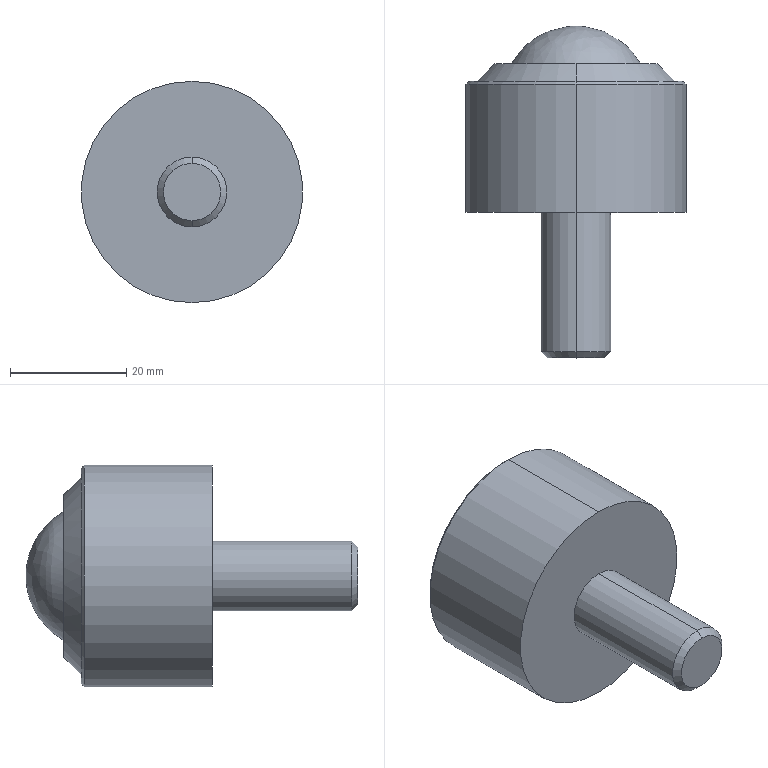Part | SolidWorks | features BaseBody 1 | 1 solid | 15 faces | box 38 x 57 x 38 mm | volume 31976 mm3 | cone 6 | plane 4 | cylinder 4 | spline 1 | commonest cylinder face diameters 12 x2 38 x2
STEP:
#1=CARTESIAN_POINT('',(0.,25.5,11.084));
#2=VERTEX_POINT('',#1);
#3=CARTESIAN_POINT('',(0.003918,25.5,-11.084));
#4=VERTEX_POINT('',#3);
#5=CARTESIAN_POINT('',(0.,25.5,11.084));
#6=CARTESIAN_POINT('',(0.3654,25.5,11.084));
#7=CARTESIAN_POINT('',(0.7294,25.5,11.066));
#8=CARTESIAN_POINT('',(1.27,25.5,11.012));
#9=CARTESIAN_POINT('',(1.45,25.5,10.99));
#10=CARTESIAN_POINT('',(1.718,25.5,10.95));
#11=CARTESIAN_POINT('',(1.851,25.5,10.929));
#12=CARTESIAN_POINT('',(1.984,25.5,10.905));
#13=CARTESIAN_POINT('',(2.072,25.5,10.888));
#14=CARTESIAN_POINT('',(2.115,25.5,10.88));
#15=CARTESIAN_POINT('',(2.526,25.5,10.799));
#16=CARTESIAN_POINT('',(2.883,25.5,10.708));
#17=CARTESIAN_POINT('',(3.405,25.5,10.549));
#18=CARTESIAN_POINT('',(3.576,25.5,10.492));
#19=CARTESIAN_POINT('',(3.83,25.5,10.402));
#20=CARTESIAN_POINT('',(3.955,25.5,10.355));
#21=CARTESIAN_POINT('',(4.1,25.5,10.298));
#22=CARTESIAN_POINT('',(4.162,25.5,10.273));
#23=CARTESIAN_POINT('',(4.203,25.5,10.256));
#24=CARTESIAN_POINT('',(4.222,25.5,10.248));
#25=CARTESIAN_POINT('',(4.592,25.5,10.095));
#26=CARTESIAN_POINT('',(4.926,25.5,9.936));
#27=CARTESIAN_POINT('',(5.403,25.5,9.679));
#28=CARTESIAN_POINT('',(5.559,25.5,9.591));
#29=CARTESIAN_POINT('',(5.786,25.5,9.454));
#30=CARTESIAN_POINT('',(5.898,25.5,9.385));
#31=CARTESIAN_POINT('',(6.027,25.5,9.302));
#32=CARTESIAN_POINT('',(6.091,25.5,9.26));
#33=CARTESIAN_POINT('',(6.118,25.5,9.242));
#34=CARTESIAN_POINT('',(6.136,25.5,9.23));
#35=CARTESIAN_POINT('',(6.144,25.5,9.225));
#36=CARTESIAN_POINT('',(6.474,25.5,9.005));
#37=CARTESIAN_POINT('',(6.774,25.5,8.78));
#38=CARTESIAN_POINT('',(7.194,25.5,8.434));
#39=CARTESIAN_POINT('',(7.33,25.5,8.316));
#40=CARTESIAN_POINT('',(7.525,25.5,8.138));
#41=CARTESIAN_POINT('',(7.622,25.5,8.048));
#42=CARTESIAN_POINT('',(7.731,25.5,7.943));
#43=CARTESIAN_POINT('',(7.785,25.5,7.89));
#44=CARTESIAN_POINT('',(7.808,25.5,7.867));
#45=CARTESIAN_POINT('',(7.823,25.5,7.852));
#46=CARTESIAN_POINT('',(7.83,25.5,7.845));
#47=CARTESIAN_POINT('',(8.112,25.5,7.562));
#48=CARTESIAN_POINT('',(8.362,25.5,7.284));
#49=CARTESIAN_POINT('',(8.704,25.5,6.864));
#50=CARTESIAN_POINT('',(8.813,25.5,6.724));
#51=CARTESIAN_POINT('',(8.969,25.5,6.513));
#52=CARTESIAN_POINT('',(9.045,25.5,6.408));
#53=CARTESIAN_POINT('',(9.13,25.5,6.285));
#54=CARTESIAN_POINT('',(9.172,25.5,6.223));
#55=CARTESIAN_POINT('',(9.19,25.5,6.197));
#56=CARTESIAN_POINT('',(9.202,25.5,6.179));
#57=CARTESIAN_POINT('',(9.206,25.5,6.172));
#58=CARTESIAN_POINT('',(9.431,25.5,5.836));
#59=CARTESIAN_POINT('',(9.622,25.5,5.513));
#60=CARTESIAN_POINT('',(9.877,25.5,5.033));
#61=CARTESIAN_POINT('',(9.956,25.5,4.874));
#62=CARTESIAN_POINT('',(10.068,25.5,4.637));
#63=CARTESIAN_POINT('',(10.122,25.5,4.519));
#64=CARTESIAN_POINT('',(10.181,25.5,4.381));
#65=CARTESIAN_POINT('',(10.211,25.5,4.312));
#66=CARTESIAN_POINT('',(10.223,25.5,4.283));
#67=CARTESIAN_POINT('',(10.231,25.5,4.263));
#68=CARTESIAN_POINT('',(10.234,25.5,4.255));
#69=CARTESIAN_POINT('',(10.388,25.5,3.884));
#70=CARTESIAN_POINT('',(10.512,25.5,3.533));
#71=CARTESIAN_POINT('',(10.668,25.5,3.015));
#72=CARTESIAN_POINT('',(10.714,25.5,2.843));
#73=CARTESIAN_POINT('',(10.778,25.5,2.588));
#74=CARTESIAN_POINT('',(10.808,25.5,2.46));
#75=CARTESIAN_POINT('',(10.84,25.5,2.311));
#76=CARTESIAN_POINT('',(10.853,25.5,2.248));
#77=CARTESIAN_POINT('',(10.862,25.5,2.206));
#78=CARTESIAN_POINT('',(10.866,25.5,2.186));
#79=CARTESIAN_POINT('',(10.907,25.5,1.981));
#80=CARTESIAN_POINT('',(10.938,25.5,1.801));
#81=CARTESIAN_POINT('',(10.978,25.5,1.533));
#82=CARTESIAN_POINT('',(10.99,25.5,1.444));
#83=CARTESIAN_POINT('',(11.012,25.5,1.265));
#84=CARTESIAN_POINT('',(11.021,25.5,1.178));
#85=CARTESIAN_POINT('',(11.066,25.5,0.7244));
#86=CARTESIAN_POINT('',(11.084,25.5,0.3682));
#87=CARTESIAN_POINT('',(11.084,25.5,-0.1753));
#88=CARTESIAN_POINT('',(11.08,25.5,-0.3557));
#89=CARTESIAN_POINT('',(11.066,25.5,-0.627));
#90=CARTESIAN_POINT('',(11.061,25.5,-0.7175));
#91=CARTESIAN_POINT('',(11.048,25.5,-0.899));
#92=CARTESIAN_POINT('',(11.04,25.5,-0.9918));
#93=CARTESIAN_POINT('',(11.013,25.5,-1.26));
#94=CARTESIAN_POINT('',(10.992,25.5,-1.439));
#95=CARTESIAN_POINT('',(10.952,25.5,-1.709));
#96=CARTESIAN_POINT('',(10.93,25.5,-1.844));
#97=CARTESIAN_POINT('',(10.902,25.5,-2.002));
#98=CARTESIAN_POINT('',(10.889,25.5,-2.071));
#99=CARTESIAN_POINT('',(10.88,25.5,-2.116));
#100=CARTESIAN_POINT('',(10.875,25.5,-2.141));
#101=CARTESIAN_POINT('',(10.804,25.5,-2.499));
#102=CARTESIAN_POINT('',(10.72,25.5,-2.838));
#103=CARTESIAN_POINT('',(10.566,25.5,-3.355));
#104=CARTESIAN_POINT('',(10.509,25.5,-3.528));
#105=CARTESIAN_POINT('',(10.416,25.5,-3.791));
#106=CARTESIAN_POINT('',(10.367,25.5,-3.923));
#107=CARTESIAN_POINT('',(10.306,25.5,-4.078));
#108=CARTESIAN_POINT('',(10.275,25.5,-4.156));
#109=CARTESIAN_POINT('',(10.261,25.5,-4.19));
#110=CARTESIAN_POINT('',(10.252,25.5,-4.212));
#111=CARTESIAN_POINT('',(10.247,25.5,-4.225));
#112=CARTESIAN_POINT('',(10.113,25.5,-4.548));
#113=CARTESIAN_POINT('',(9.966,25.5,-4.865));
#114=CARTESIAN_POINT('',(9.711,25.5,-5.345));
#115=CARTESIAN_POINT('',(9.621,25.5,-5.506));
#116=CARTESIAN_POINT('',(9.477,25.5,-5.749));
#117=CARTESIAN_POINT('',(9.402,25.5,-5.87));
#118=CARTESIAN_POINT('',(9.311,25.5,-6.013));
#119=CARTESIAN_POINT('',(9.265,25.5,-6.084));
#120=CARTESIAN_POINT('',(9.245,25.5,-6.115));
#121=CARTESIAN_POINT('',(9.231,25.5,-6.135));
#122=CARTESIAN_POINT('',(9.223,25.5,-6.147));
#123=CARTESIAN_POINT('',(9.029,25.5,-6.437));
#124=CARTESIAN_POINT('',(8.823,25.5,-6.719));
#125=CARTESIAN_POINT('',(8.48,25.5,-7.139));
#126=CARTESIAN_POINT('',(8.361,25.5,-7.279));
#127=CARTESIAN_POINT('',(8.173,25.5,-7.488));
#128=CARTESIAN_POINT('',(8.076,25.5,-7.592));
#129=CARTESIAN_POINT('',(7.96,25.5,-7.713));
#130=CARTESIAN_POINT('',(7.901,25.5,-7.773));
#131=CARTESIAN_POINT('',(7.876,25.5,-7.799));
#132=CARTESIAN_POINT('',(7.859,25.5,-7.816));
#133=CARTESIAN_POINT('',(7.849,25.5,-7.826));
#134=CARTESIAN_POINT('',(7.599,25.5,-8.076));
#135=CARTESIAN_POINT('',(7.34,25.5,-8.313));
#136=CARTESIAN_POINT('',(6.921,25.5,-8.66));
#137=CARTESIAN_POINT('',(6.776,25.5,-8.773));
#138=CARTESIAN_POINT('',(6.552,25.5,-8.94));
#139=CARTESIAN_POINT('',(6.438,25.5,-9.023));
#140=CARTESIAN_POINT('',(6.302,25.5,-9.118));
#141=CARTESIAN_POINT('',(6.243,25.5,-9.159));
#142=CARTESIAN_POINT('',(6.203,25.5,-9.185));
#143=CARTESIAN_POINT('',(6.181,25.5,-9.2));
#144=CARTESIAN_POINT('',(5.874,25.5,-9.406));
#145=CARTESIAN_POINT('',(5.569,25.5,-9.59));
#146=CARTESIAN_POINT('',(5.089,25.5,-9.848));
#147=CARTESIAN_POINT('',(4.926,25.5,-9.931));
#148=CARTESIAN_POINT('',(4.674,25.5,-10.05));
#149=CARTESIAN_POINT('',(4.547,25.5,-10.109));
#150=CARTESIAN_POINT('',(4.396,25.5,-10.175));
#151=CARTESIAN_POINT('',(4.331,25.5,-10.202));
#152=CARTESIAN_POINT('',(4.288,25.5,-10.221));
#153=CARTESIAN_POINT('',(4.265,25.5,-10.231));
#154=CARTESIAN_POINT('',(3.919,25.5,-10.374));
#155=CARTESIAN_POINT('',(3.583,25.5,-10.495));
#156=CARTESIAN_POINT('',(3.064,25.5,-10.653));
#157=CARTESIAN_POINT('',(2.888,25.5,-10.702));
#158=CARTESIAN_POINT('',(2.622,25.5,-10.77));
#159=CARTESIAN_POINT('',(2.488,25.5,-10.802));
#160=CARTESIAN_POINT('',(2.353,25.5,-10.831));
#161=CARTESIAN_POINT('',(2.263,25.5,-10.85));
#162=CARTESIAN_POINT('',(2.216,25.5,-10.86));
#163=CARTESIAN_POINT('',(1.465,25.5,-11.01));
#164=CARTESIAN_POINT('',(0.7373,25.5,-11.084));
#165=CARTESIAN_POINT('',(0.003918,25.5,-11.084));
#166=B_SPLINE_CURVE_WITH_KNOTS('',3,(#5,#6,#7,#8,#9,#10,#11,#12,#13,#14,#15,#16,#17,#18,#19,#20,#21,#22,#23,#24,#25,#26,#27,#28,#29,#30,#31,#32,#33,#34,#35,#36,#37,#38,#39,#40,#41,#42,#43,#44,#45,#46,#47,#48,#49,#50,#51,#52,#53,#54,#55,#56,#57,#58,#59,#60,#61,#62,#63,#64,#65,#66,#67,#68,#69,#70,#71,#72,#73,#74,#75,#76,#77,#78,#79,#80,#81,#82,#83,#84,#85,#86,#87,#88,#89,#90,#91,#92,#93,#94,#95,#96,#97,#98,#99,#100,#101,#102,#103,#104,#105,#106,#107,#108,#109,#110,#111,#112,#113,#114,#115,#116,#117,#118,#119,#120,#121,#122,#123,#124,#125,#126,#127,#128,#129,#130,#131,#132,#133,#134,#135,#136,#137,#138,#139,#140,#141,#142,#143,#144,#145,#146,#147,#148,#149,#150,#151,#152,#153,#154,#155,#156,#157,#158,#159,#160,#161,#162,#163,#164,#165),.UNSPECIFIED.,.F.,.F.,(4,2,2,1,2,2,2,2,1,1,2,2,2,2,1,1,1,2,2,2,2,1,1,1,2,2,2,2,1,1,1,2,2,2,2,1,1,1,2,2,2,2,1,1,2,2,2,2,2,2,2,2,2,2,1,1,2,2,2,2,1,1,1,2,2,2,2,1,1,1,2,2,2,2,1,1,1,2,2,2,2,1,1,2,2,2,2,1,1,2,2,2,2,1,2,2,4),(0.,0.03125,0.04687,0.05469,0.05859,0.0625,0.09375,0.1094,0.1172,0.1211,0.123,0.125,0.1562,0.1719,0.1797,0.1836,0.1855,0.1865,0.1875,0.2187,0.2344,0.2422,0.2461,0.248,0.249,0.25,0.2812,0.2969,0.3047,0.3086,0.3105,0.3115,0.3125,0.3437,0.3594,0.3672,0.3711,0.373,0.374,0.375,0.4062,0.4219,0.4297,0.4336,0.4355,0.4375,0.4531,0.4609,0.4687,0.5,0.5156,0.5234,0.5312,0.5469,0.5547,0.5586,0.5605,0.5625,0.5937,0.6094,0.6172,0.6211,0.623,0.624,0.625,0.6562,0.6719,0.6797,0.6836,0.6855,0.6865,0.6875,0.7187,0.7344,0.7422,0.7461,0.748,0.749,0.75,0.7812,0.7969,0.8047,0.8086,0.8105,0.8125,0.8437,0.8594,0.8672,0.8711,0.873,0.875,0.9062,0.9219,0.9297,0.9336,0.9375,1.),.UNSPECIFIED.);
#167=EDGE_CURVE('',#2,#4,#166,.T.);
#168=ORIENTED_EDGE('',*,*,#167,.T.);
#169=CARTESIAN_POINT('',(0.003918,25.5,-11.084));
#170=CARTESIAN_POINT('',(-0.3607,25.5,-11.084));
#171=CARTESIAN_POINT('',(-0.7241,25.5,-11.066));
#172=CARTESIAN_POINT('',(-1.264,25.5,-11.013));
#173=CARTESIAN_POINT('',(-1.443,25.5,-10.991));
#174=CARTESIAN_POINT('',(-1.711,25.5,-10.951));
#175=CARTESIAN_POINT('',(-1.844,25.5,-10.93));
#176=CARTESIAN_POINT('',(-1.976,25.5,-10.906));
#177=CARTESIAN_POINT('',(-2.065,25.5,-10.89));
#178=CARTESIAN_POINT('',(-2.107,25.5,-10.882));
#179=CARTESIAN_POINT('',(-2.518,25.5,-10.8));
#180=CARTESIAN_POINT('',(-2.875,25.5,-10.711));
#181=CARTESIAN_POINT('',(-3.396,25.5,-10.552));
#182=CARTESIAN_POINT('',(-3.568,25.5,-10.495));
#183=CARTESIAN_POINT('',(-3.821,25.5,-10.405));
#184=CARTESIAN_POINT('',(-3.946,25.5,-10.358));
#185=CARTESIAN_POINT('',(-4.091,25.5,-10.301));
#186=CARTESIAN_POINT('',(-4.153,25.5,-10.276));
#187=CARTESIAN_POINT('',(-4.194,25.5,-10.26));
#188=CARTESIAN_POINT('',(-4.213,25.5,-10.252));
#189=CARTESIAN_POINT('',(-4.585,25.5,-10.098));
#190=CARTESIAN_POINT('',(-4.919,25.5,-9.939));
#191=CARTESIAN_POINT('',(-5.399,25.5,-9.682));
#192=CARTESIAN_POINT('',(-5.555,25.5,-9.593));
#193=CARTESIAN_POINT('',(-5.783,25.5,-9.456));
#194=CARTESIAN_POINT('',(-5.896,25.5,-9.386));
#195=CARTESIAN_POINT('',(-6.025,25.5,-9.303));
#196=CARTESIAN_POINT('',(-6.08,25.5,-9.267));
#197=CARTESIAN_POINT('',(-6.116,25.5,-9.243));
#198=CARTESIAN_POINT('',(-6.133,25.5,-9.233));
#199=CARTESIAN_POINT('',(-6.471,25.5,-9.007));
#200=CARTESIAN_POINT('',(-6.77,25.5,-8.784));
#201=CARTESIAN_POINT('',(-7.188,25.5,-8.439));
#202=CARTESIAN_POINT('',(-7.323,25.5,-8.322));
#203=CARTESIAN_POINT('',(-7.518,25.5,-8.145));
#204=CARTESIAN_POINT('',(-7.614,25.5,-8.055));
#205=CARTESIAN_POINT('',(-7.723,25.5,-7.95));
#206=CARTESIAN_POINT('',(-7.777,25.5,-7.898));
#207=CARTESIAN_POINT('',(-7.799,25.5,-7.875));
#208=CARTESIAN_POINT('',(-7.815,25.5,-7.86));
#209=CARTESIAN_POINT('',(-7.821,25.5,-7.854));
#210=CARTESIAN_POINT('',(-8.106,25.5,-7.57));
#211=CARTESIAN_POINT('',(-8.357,25.5,-7.29));
#212=CARTESIAN_POINT('',(-8.701,25.5,-6.868));
#213=CARTESIAN_POINT('',(-8.811,25.5,-6.727));
#214=CARTESIAN_POINT('',(-8.967,25.5,-6.515));
#215=CARTESIAN_POINT('',(-9.043,25.5,-6.41));
#216=CARTESIAN_POINT('',(-9.129,25.5,-6.286));
#217=CARTESIAN_POINT('',(-9.171,25.5,-6.224));
#218=CARTESIAN_POINT('',(-9.189,25.5,-6.198));
#219=CARTESIAN_POINT('',(-9.201,25.5,-6.18));
#220=CARTESIAN_POINT('',(-9.206,25.5,-6.173));
#221=CARTESIAN_POINT('',(-9.43,25.5,-5.838));
#222=CARTESIAN_POINT('',(-9.62,25.5,-5.516));
#223=CARTESIAN_POINT('',(-9.874,25.5,-5.039));
#224=CARTESIAN_POINT('',(-9.953,25.5,-4.881));
#225=CARTESIAN_POINT('',(-10.064,25.5,-4.645));
#226=CARTESIAN_POINT('',(-10.118,25.5,-4.527));
#227=CARTESIAN_POINT('',(-10.178,25.5,-4.39));
#228=CARTESIAN_POINT('',(-10.207,25.5,-4.322));
#229=CARTESIAN_POINT('',(-10.219,25.5,-4.292));
#230=CARTESIAN_POINT('',(-10.227,25.5,-4.273));
#231=CARTESIAN_POINT('',(-10.231,25.5,-4.265));
#232=CARTESIAN_POINT('',(-10.385,25.5,-3.893));
#233=CARTESIAN_POINT('',(-10.509,25.5,-3.542));
#234=CARTESIAN_POINT('',(-10.665,25.5,-3.023));
#235=CARTESIAN_POINT('',(-10.712,25.5,-2.851));
#236=CARTESIAN_POINT('',(-10.776,25.5,-2.595));
#237=CARTESIAN_POINT('',(-10.806,25.5,-2.467));
#238=CARTESIAN_POINT('',(-10.839,25.5,-2.318));
#239=CARTESIAN_POINT('',(-10.852,25.5,-2.255));
#240=CARTESIAN_POINT('',(-10.861,25.5,-2.212));
#241=CARTESIAN_POINT('',(-10.865,25.5,-2.193));
#242=CARTESIAN_POINT('',(-10.905,25.5,-1.989));
#243=CARTESIAN_POINT('',(-10.937,25.5,-1.81));
#244=CARTESIAN_POINT('',(-10.976,25.5,-1.542));
#245=CARTESIAN_POINT('',(-10.995,25.5,-1.409));
#246=CARTESIAN_POINT('',(-11.01,25.5,-1.276));
#247=CARTESIAN_POINT('',(-11.02,25.5,-1.188));
#248=CARTESIAN_POINT('',(-11.025,25.5,-1.145));
#249=CARTESIAN_POINT('',(-11.066,25.5,-0.7339));
#250=CARTESIAN_POINT('',(-11.083,25.5,-0.3748));
#251=CARTESIAN_POINT('',(-11.084,25.5,0.1704));
#252=CARTESIAN_POINT('',(-11.08,25.5,0.3515));
#253=CARTESIAN_POINT('',(-11.067,25.5,0.6236));
#254=CARTESIAN_POINT('',(-11.058,25.5,0.7598));
#255=CARTESIAN_POINT('',(-11.048,25.5,0.8965));
#256=CARTESIAN_POINT('',(-11.04,25.5,0.9878));
#257=CARTESIAN_POINT('',(-11.035,25.5,1.035));
#258=CARTESIAN_POINT('',(-11.014,25.5,1.257));
#259=CARTESIAN_POINT('',(-10.992,25.5,1.434));
#260=CARTESIAN_POINT('',(-10.953,25.5,1.702));
#261=CARTESIAN_POINT('',(-10.931,25.5,1.836));
#262=CARTESIAN_POINT('',(-10.903,25.5,1.993));
#263=CARTESIAN_POINT('',(-10.891,25.5,2.061));
#264=CARTESIAN_POINT('',(-10.882,25.5,2.106));
#265=CARTESIAN_POINT('',(-10.877,25.5,2.13));
#266=CARTESIAN_POINT('',(-10.806,25.5,2.49));
#267=CARTESIAN_POINT('',(-10.723,25.5,2.831));
#268=CARTESIAN_POINT('',(-10.567,25.5,3.35));
#269=CARTESIAN_POINT('',(-10.51,25.5,3.524));
#270=CARTESIAN_POINT('',(-10.417,25.5,3.788));
#271=CARTESIAN_POINT('',(-10.368,25.5,3.921));
#272=CARTESIAN_POINT('',(-10.307,25.5,4.077));
#273=CARTESIAN_POINT('',(-10.275,25.5,4.155));
#274=CARTESIAN_POINT('',(-10.262,25.5,4.189));
#275=CARTESIAN_POINT('',(-10.252,25.5,4.212));
#276=CARTESIAN_POINT('',(-10.247,25.5,4.224));
#277=CARTESIAN_POINT('',(-10.114,25.5,4.546));
#278=CARTESIAN_POINT('',(-9.967,25.5,4.861));
#279=CARTESIAN_POINT('',(-9.715,25.5,5.339));
#280=CARTESIAN_POINT('',(-9.625,25.5,5.5));
#281=CARTESIAN_POINT('',(-9.482,25.5,5.741));
#282=CARTESIAN_POINT('',(-9.408,25.5,5.862));
#283=CARTESIAN_POINT('',(-9.317,25.5,6.004));
#284=CARTESIAN_POINT('',(-9.271,25.5,6.075));
#285=CARTESIAN_POINT('',(-9.251,25.5,6.105));
#286=CARTESIAN_POINT('',(-9.237,25.5,6.125));
#287=CARTESIAN_POINT('',(-9.23,25.5,6.137));
#288=CARTESIAN_POINT('',(-9.035,25.5,6.428));
#289=CARTESIAN_POINT('',(-8.828,25.5,6.712));
#290=CARTESIAN_POINT('',(-8.485,25.5,7.134));
#291=CARTESIAN_POINT('',(-8.365,25.5,7.274));
#292=CARTESIAN_POINT('',(-8.176,25.5,7.484));
#293=CARTESIAN_POINT('',(-8.079,25.5,7.589));
#294=CARTESIAN_POINT('',(-7.963,25.5,7.71));
#295=CARTESIAN_POINT('',(-7.904,25.5,7.771));
#296=CARTESIAN_POINT('',(-7.878,25.5,7.797));
#297=CARTESIAN_POINT('',(-7.861,25.5,7.814));
#298=CARTESIAN_POINT('',(-7.851,25.5,7.824));
#299=CARTESIAN_POINT('',(-7.602,25.5,8.073));
#300=CARTESIAN_POINT('',(-7.343,25.5,8.31));
#301=CARTESIAN_POINT('',(-6.926,25.5,8.656));
#302=CARTESIAN_POINT('',(-6.781,25.5,8.769));
#303=CARTESIAN_POINT('',(-6.558,25.5,8.936));
#304=CARTESIAN_POINT('',(-6.444,25.5,9.019));
#305=CARTESIAN_POINT('',(-6.309,25.5,9.114));
#306=CARTESIAN_POINT('',(-6.25,25.5,9.154));
#307=CARTESIAN_POINT('',(-6.21,25.5,9.181));
#308=CARTESIAN_POINT('',(-6.189,25.5,9.195));
#309=CARTESIAN_POINT('',(-5.881,25.5,9.401));
#310=CARTESIAN_POINT('',(-5.577,25.5,9.585));
#311=CARTESIAN_POINT('',(-5.097,25.5,9.844));
#312=CARTESIAN_POINT('',(-4.934,25.5,9.927));
#313=CARTESIAN_POINT('',(-4.683,25.5,10.047));
#314=CARTESIAN_POINT('',(-4.556,25.5,10.105));
#315=CARTESIAN_POINT('',(-4.405,25.5,10.171));
#316=CARTESIAN_POINT('',(-4.34,25.5,10.199));
#317=CARTESIAN_POINT('',(-4.296,25.5,10.217));
#318=CARTESIAN_POINT('',(-4.273,25.5,10.227));
#319=CARTESIAN_POINT('',(-3.926,25.5,10.371));
#320=CARTESIAN_POINT('',(-3.589,25.5,10.493));
#321=CARTESIAN_POINT('',(-3.069,25.5,10.652));
#322=CARTESIAN_POINT('',(-2.893,25.5,10.701));
#323=CARTESIAN_POINT('',(-2.626,25.5,10.769));
#324=CARTESIAN_POINT('',(-2.491,25.5,10.801));
#325=CARTESIAN_POINT('',(-2.356,25.5,10.831));
#326=CARTESIAN_POINT('',(-2.265,25.5,10.85));
#327=CARTESIAN_POINT('',(-2.218,25.5,10.86));
#328=CARTESIAN_POINT('',(-1.465,25.5,11.01));
#329=CARTESIAN_POINT('',(-0.7354,25.5,11.084));
#330=CARTESIAN_POINT('',(0.,25.5,11.084));
#331=B_SPLINE_CURVE_WITH_KNOTS('',3,(#169,#170,#171,#172,#173,#174,#175,#176,#177,#178,#179,#180,#181,#182,#183,#184,#185,#186,#187,#188,#189,#190,#191,#192,#193,#194,#195,#196,#197,#198,#199,#200,#201,#202,#203,#204,#205,#206,#207,#208,#209,#210,#211,#212,#213,#214,#215,#216,#217,#218,#219,#220,#221,#222,#223,#224,#225,#226,#227,#228,#229,#230,#231,#232,#233,#234,#235,#236,#237,#238,#239,#240,#241,#242,#243,#244,#245,#246,#247,#248,#249,#250,#251,#252,#253,#254,#255,#256,#257,#258,#259,#260,#261,#262,#263,#264,#265,#266,#267,#268,#269,#270,#271,#272,#273,#274,#275,#276,#277,#278,#279,#280,#281,#282,#283,#284,#285,#286,#287,#288,#289,#290,#291,#292,#293,#294,#295,#296,#297,#298,#299,#300,#301,#302,#303,#304,#305,#306,#307,#308,#309,#310,#311,#312,#313,#314,#315,#316,#317,#318,#319,#320,#321,#322,#323,#324,#325,#326,#327,#328,#329,#330),.UNSPECIFIED.,.F.,.F.,(4,2,2,1,2,2,2,2,1,1,2,2,2,2,1,1,2,2,2,2,1,1,1,2,2,2,2,1,1,1,2,2,2,2,1,1,1,2,2,2,2,1,1,2,2,2,1,2,2,2,2,1,2,2,2,1,1,2,2,2,2,1,1,1,2,2,2,2,1,1,1,2,2,2,2,1,1,1,2,2,2,2,1,1,2,2,2,2,1,1,2,2,2,2,1,2,2,4),(0.,0.03125,0.04687,0.05469,0.05859,0.0625,0.09375,0.1094,0.1172,0.1211,0.123,0.125,0.1563,0.1719,0.1797,0.1836,0.1855,0.1875,0.2188,0.2344,0.2422,0.2461,0.248,0.249,0.25,0.2813,0.2969,0.3047,0.3086,0.3105,0.3115,0.3125,0.3438,0.3594,0.3672,0.3711,0.373,0.374,0.375,0.4063,0.4219,0.4297,0.4336,0.4355,0.4375,0.4531,0.4609,0.4648,0.4688,0.5,0.5156,0.5234,0.5273,0.5313,0.5469,0.5547,0.5586,0.5605,0.5625,0.5938,0.6094,0.6172,0.6211,0.623,0.624,0.625,0.6563,0.6719,0.6797,0.6836,0.6855,0.6865,0.6875,0.7188,0.7344,0.7422,0.7461,0.748,0.749,0.75,0.7813,0.7969,0.8047,0.8086,0.8105,0.8125,0.8438,0.8594,0.8672,0.8711,0.873,0.875,0.9063,0.9219,0.9297,0.9336,0.9375,1.),.UNSPECIFIED.);
#332=EDGE_CURVE('',#4,#2,#331,.T.);
#333=ORIENTED_EDGE('',*,*,#332,.T.);
#334=EDGE_LOOP('',(#168,#333));
#335=FACE_OUTER_BOUND('',#334,.T.);
#336=CARTESIAN_POINT('',(-11.175,22.179,5.304));
#337=CARTESIAN_POINT('',(-11.175,26.959,2.709));
#338=CARTESIAN_POINT('',(-11.175,26.952,-2.73));
#339=CARTESIAN_POINT('',(-11.175,22.164,-5.311));
#340=CARTESIAN_POINT('',(-5.695,27.019,14.222));
#341=CARTESIAN_POINT('',(-5.695,39.837,7.265));
#342=CARTESIAN_POINT('',(-5.695,39.817,-7.32));
#343=CARTESIAN_POINT('',(-5.695,26.981,-14.242));
#344=CARTESIAN_POINT('',(5.836,26.995,14.177));
#345=CARTESIAN_POINT('',(5.836,39.773,7.242));
#346=CARTESIAN_POINT('',(5.836,39.753,-7.297));
#347=CARTESIAN_POINT('',(5.836,26.957,-14.198));
#348=CARTESIAN_POINT('',(11.227,22.132,5.218));
#349=CARTESIAN_POINT('',(11.227,26.835,2.665));
#350=CARTESIAN_POINT('',(11.227,26.828,-2.686));
#351=CARTESIAN_POINT('',(11.227,22.118,-5.225));
#352=(BOUNDED_SURFACE()B_SPLINE_SURFACE(3,3,((#336,#337,#338,#339),(#340,#341,#342,#343),(#344,#345,#346,#347),(#348,#349,#350,#351)),.UNSPECIFIED.,.F.,.F.,.F.)B_SPLINE_SURFACE_WITH_KNOTS((4,4),(4,4),(0.,1.),(0.,1.),.UNSPECIFIED.)GEOMETRIC_REPRESENTATION_ITEM()RATIONAL_B_SPLINE_SURFACE(((1.,0.6506,0.6506,1.),(0.6475,0.4213,0.4213,0.6475),(0.6475,0.4213,0.4213,0.6475),(1.,0.6506,0.6506,1.)))REPRESENTATION_ITEM('')SURFACE());
#353=ADVANCED_FACE('',(#335),#352,.T.);
#354=ORIENTED_EDGE('',*,*,#167,.F.);
#355=ORIENTED_EDGE('',*,*,#332,.F.);
#356=EDGE_LOOP('',(#354,#355));
#357=FACE_BOUND('',#356,.T.);
#358=CARTESIAN_POINT('',(0.,25.5,-14.));
#359=VERTEX_POINT('',#358);
#360=CARTESIAN_POINT('',(0.,25.5,14.));
#361=VERTEX_POINT('',#360);
#362=CARTESIAN_POINT('',(0.,25.5,0.));
#363=DIRECTION('',(0.,-1.,0.));
#364=DIRECTION('',(0.,0.,-1.));
#365=AXIS2_PLACEMENT_3D('',#362,#363,#364);
#366=CIRCLE('',#365,14.);
#367=EDGE_CURVE('',#359,#361,#366,.T.);
#368=ORIENTED_EDGE('',*,*,#367,.F.);
#369=CARTESIAN_POINT('',(0.,25.5,0.));
#370=DIRECTION('',(0.,-1.,0.));
#371=DIRECTION('',(0.,0.,-1.));
#372=AXIS2_PLACEMENT_3D('',#369,#370,#371);
#373=CIRCLE('',#372,14.);
#374=EDGE_CURVE('',#361,#359,#373,.T.);
#375=ORIENTED_EDGE('',*,*,#374,.F.);
#376=EDGE_LOOP('',(#368,#375));
#377=FACE_OUTER_BOUND('',#376,.T.);
#378=CARTESIAN_POINT('',(-14.,25.5,0.));
#379=DIRECTION('',(0.,-1.,0.));
#380=DIRECTION('',(0.,0.,-1.));
#381=AXIS2_PLACEMENT_3D('',#378,#379,#380);
#382=PLANE('',#381);
#383=ADVANCED_FACE('',(#357,#377),#382,.F.);
#384=CARTESIAN_POINT('',(0.,-25.,4.927));
#385=VERTEX_POINT('',#384);
#386=CARTESIAN_POINT('',(0.,-25.,-4.927));
#387=VERTEX_POINT('',#386);
#388=CARTESIAN_POINT('',(0.,-25.,0.));
#389=DIRECTION('',(0.,1.,0.));
#390=DIRECTION('',(0.,0.,1.));
#391=AXIS2_PLACEMENT_3D('',#388,#389,#390);
#392=CIRCLE('',#391,4.927);
#393=EDGE_CURVE('',#385,#387,#392,.T.);
#394=ORIENTED_EDGE('',*,*,#393,.F.);
#395=CARTESIAN_POINT('',(0.,-25.,0.));
#396=DIRECTION('',(0.,1.,0.));
#397=DIRECTION('',(0.,0.,1.));
#398=AXIS2_PLACEMENT_3D('',#395,#396,#397);
#399=CIRCLE('',#398,4.927);
#400=EDGE_CURVE('',#387,#385,#399,.T.);
#401=ORIENTED_EDGE('',*,*,#400,.F.);
#402=EDGE_LOOP('',(#394,#401));
#403=FACE_OUTER_BOUND('',#402,.T.);
#404=CARTESIAN_POINT('',(0.,-25.,0.));
#405=DIRECTION('',(0.,1.,0.));
#406=DIRECTION('',(1.,0.,0.));
#407=AXIS2_PLACEMENT_3D('',#404,#405,#406);
#408=PLANE('',#407);
#409=ADVANCED_FACE('',(#403),#408,.F.);
#410=CARTESIAN_POINT('',(0.,22.5,17.));
#411=VERTEX_POINT('',#410);
#412=CARTESIAN_POINT('',(0.,22.5,17.));
#413=DIRECTION('',(0.,-0.7071,0.7071));
#414=VECTOR('',#413,1000.);
#415=LINE('',#412,#414);
#416=EDGE_CURVE('',#361,#411,#415,.T.);
#417=ORIENTED_EDGE('',*,*,#416,.F.);
#418=ORIENTED_EDGE('',*,*,#374,.T.);
#419=CARTESIAN_POINT('',(0.,22.5,-17.));
#420=VERTEX_POINT('',#419);
#421=CARTESIAN_POINT('',(0.,22.5,-17.));
#422=DIRECTION('',(0.,-0.7071,-0.7071));
#423=VECTOR('',#422,1000.);
#424=LINE('',#421,#423);
#425=EDGE_CURVE('',#359,#420,#424,.T.);
#426=ORIENTED_EDGE('',*,*,#425,.T.);
#427=CARTESIAN_POINT('',(0.,22.5,0.));
#428=DIRECTION('',(0.,1.,0.));
#429=DIRECTION('',(0.,0.,-1.));
#430=AXIS2_PLACEMENT_3D('',#427,#428,#429);
#431=CIRCLE('',#430,17.);
#432=EDGE_CURVE('',#420,#411,#431,.T.);
#433=ORIENTED_EDGE('',*,*,#432,.T.);
#434=EDGE_LOOP('',(#417,#418,#426,#433));
#435=FACE_OUTER_BOUND('',#434,.T.);
#436=CARTESIAN_POINT('',(0.,22.5,0.));
#437=DIRECTION('',(0.,-1.,0.));
#438=DIRECTION('',(0.,0.,-1.));
#439=AXIS2_PLACEMENT_3D('',#436,#437,#438);
#440=CONICAL_SURFACE('',#439,17.,0.7854);
#441=ADVANCED_FACE('',(#435),#440,.T.);
#442=CARTESIAN_POINT('',(0.,-23.927,-6.));
#443=VERTEX_POINT('',#442);
#444=CARTESIAN_POINT('',(0.,-23.926,-6.));
#445=DIRECTION('',(0.,0.7071,-0.7071));
#446=VECTOR('',#445,1000.);
#447=LINE('',#444,#446);
#448=EDGE_CURVE('',#387,#443,#447,.T.);
#449=ORIENTED_EDGE('',*,*,#448,.F.);
#450=ORIENTED_EDGE('',*,*,#400,.T.);
#451=CARTESIAN_POINT('',(0.,-23.927,6.));
#452=VERTEX_POINT('',#451);
#453=CARTESIAN_POINT('',(0.,-23.926,6.));
#454=DIRECTION('',(0.,0.7071,0.7071));
#455=VECTOR('',#454,1000.);
#456=LINE('',#453,#455);
#457=EDGE_CURVE('',#385,#452,#456,.T.);
#458=ORIENTED_EDGE('',*,*,#457,.T.);
#459=CARTESIAN_POINT('',(0.,-23.927,0.));
#460=DIRECTION('',(0.,1.,0.));
#461=DIRECTION('',(0.,0.,-1.));
#462=AXIS2_PLACEMENT_3D('',#459,#460,#461);
#463=CIRCLE('',#462,6.);
#464=EDGE_CURVE('',#443,#452,#463,.T.);
#465=ORIENTED_EDGE('',*,*,#464,.F.);
#466=EDGE_LOOP('',(#449,#450,#458,#465));
#467=FACE_OUTER_BOUND('',#466,.T.);
#468=CARTESIAN_POINT('',(0.,-23.926,0.));
#469=DIRECTION('',(0.,1.,0.));
#470=DIRECTION('',(0.,0.,1.));
#471=AXIS2_PLACEMENT_3D('',#468,#469,#470);
#472=CONICAL_SURFACE('',#471,6.,0.7854);
#473=ADVANCED_FACE('',(#467),#472,.T.);
#474=ORIENTED_EDGE('',*,*,#432,.F.);
#475=CARTESIAN_POINT('',(0.,22.5,0.));
#476=DIRECTION('',(0.,1.,0.));
#477=DIRECTION('',(0.,0.,-1.));
#478=AXIS2_PLACEMENT_3D('',#475,#476,#477);
#479=CIRCLE('',#478,17.);
#480=EDGE_CURVE('',#411,#420,#479,.T.);
#481=ORIENTED_EDGE('',*,*,#480,.F.);
#482=EDGE_LOOP('',(#474,#481));
#483=FACE_BOUND('',#482,.T.);
#484=CARTESIAN_POINT('',(0.,22.5,-18.5));
#485=VERTEX_POINT('',#484);
#486=CARTESIAN_POINT('',(0.,22.5,18.5));
#487=VERTEX_POINT('',#486);
#488=CARTESIAN_POINT('',(0.,22.5,0.));
#489=DIRECTION('',(0.,-1.,0.));
#490=DIRECTION('',(0.,0.,-1.));
#491=AXIS2_PLACEMENT_3D('',#488,#489,#490);
#492=CIRCLE('',#491,18.5);
#493=EDGE_CURVE('',#485,#487,#492,.T.);
#494=ORIENTED_EDGE('',*,*,#493,.F.);
#495=CARTESIAN_POINT('',(0.,22.5,0.));
#496=DIRECTION('',(0.,-1.,0.));
#497=DIRECTION('',(0.,0.,-1.));
#498=AXIS2_PLACEMENT_3D('',#495,#496,#497);
#499=CIRCLE('',#498,18.5);
#500=EDGE_CURVE('',#487,#485,#499,.T.);
#501=ORIENTED_EDGE('',*,*,#500,.F.);
#502=EDGE_LOOP('',(#494,#501));
#503=FACE_OUTER_BOUND('',#502,.T.);
#504=CARTESIAN_POINT('',(-18.5,22.5,0.));
#505=DIRECTION('',(0.,-1.,0.));
#506=DIRECTION('',(0.,0.,-1.));
#507=AXIS2_PLACEMENT_3D('',#504,#505,#506);
#508=PLANE('',#507);
#509=ADVANCED_FACE('',(#483,#503),#508,.F.);
#510=CARTESIAN_POINT('',(0.,0.,6.));
#511=VERTEX_POINT('',#510);
#512=CARTESIAN_POINT('',(0.,32.,6.));
#513=DIRECTION('',(0.,-1.,0.));
#514=VECTOR('',#513,1000.);
#515=LINE('',#512,#514);
#516=EDGE_CURVE('',#511,#452,#515,.T.);
#517=ORIENTED_EDGE('',*,*,#516,.F.);
#518=CARTESIAN_POINT('',(0.,0.,-6.));
#519=VERTEX_POINT('',#518);
#520=CARTESIAN_POINT('',(0.,0.,0.));
#521=DIRECTION('',(0.,-1.,0.));
#522=DIRECTION('',(0.,0.,-1.));
#523=AXIS2_PLACEMENT_3D('',#520,#521,#522);
#524=CIRCLE('',#523,6.);
#525=EDGE_CURVE('',#511,#519,#524,.T.);
#526=ORIENTED_EDGE('',*,*,#525,.T.);
#527=CARTESIAN_POINT('',(0.,32.,-6.));
#528=DIRECTION('',(0.,-1.,0.));
#529=VECTOR('',#528,1000.);
#530=LINE('',#527,#529);
#531=EDGE_CURVE('',#519,#443,#530,.T.);
#532=ORIENTED_EDGE('',*,*,#531,.T.);
#533=ORIENTED_EDGE('',*,*,#464,.T.);
#534=EDGE_LOOP('',(#517,#526,#532,#533));
#535=FACE_OUTER_BOUND('',#534,.T.);
#536=CARTESIAN_POINT('',(0.,32.,0.));
#537=DIRECTION('',(0.,-1.,0.));
#538=DIRECTION('',(0.,0.,-1.));
#539=AXIS2_PLACEMENT_3D('',#536,#537,#538);
#540=CYLINDRICAL_SURFACE('',#539,6.);
#541=ADVANCED_FACE('',(#535),#540,.T.);
#542=CARTESIAN_POINT('',(0.,22.,19.));
#543=VERTEX_POINT('',#542);
#544=CARTESIAN_POINT('',(0.,22.,19.));
#545=DIRECTION('',(0.,-0.7071,0.7071));
#546=VECTOR('',#545,1000.);
#547=LINE('',#544,#546);
#548=EDGE_CURVE('',#487,#543,#547,.T.);
#549=ORIENTED_EDGE('',*,*,#548,.F.);
#550=ORIENTED_EDGE('',*,*,#500,.T.);
#551=CARTESIAN_POINT('',(0.,22.,-19.));
#552=VERTEX_POINT('',#551);
#553=CARTESIAN_POINT('',(0.,22.,-19.));
#554=DIRECTION('',(0.,-0.7071,-0.7071));
#555=VECTOR('',#554,1000.);
#556=LINE('',#553,#555);
#557=EDGE_CURVE('',#485,#552,#556,.T.);
#558=ORIENTED_EDGE('',*,*,#557,.T.);
#559=CARTESIAN_POINT('',(0.,22.,0.));
#560=DIRECTION('',(0.,-1.,0.));
#561=DIRECTION('',(0.,0.,-1.));
#562=AXIS2_PLACEMENT_3D('',#559,#560,#561);
#563=CIRCLE('',#562,19.);
#564=EDGE_CURVE('',#543,#552,#563,.T.);
#565=ORIENTED_EDGE('',*,*,#564,.F.);
#566=EDGE_LOOP('',(#549,#550,#558,#565));
#567=FACE_OUTER_BOUND('',#566,.T.);
#568=CARTESIAN_POINT('',(0.,22.,0.));
#569=DIRECTION('',(0.,-1.,0.));
#570=DIRECTION('',(0.,0.,-1.));
#571=AXIS2_PLACEMENT_3D('',#568,#569,#570);
#572=CONICAL_SURFACE('',#571,19.,0.7854);
#573=ADVANCED_FACE('',(#567),#572,.T.);
#574=CARTESIAN_POINT('',(0.,0.,0.));
#575=DIRECTION('',(0.,-1.,0.));
#576=DIRECTION('',(0.,0.,-1.));
#577=AXIS2_PLACEMENT_3D('',#574,#575,#576);
#578=CIRCLE('',#577,6.);
#579=EDGE_CURVE('',#519,#511,#578,.T.);
#580=ORIENTED_EDGE('',*,*,#579,.F.);
#581=ORIENTED_EDGE('',*,*,#525,.F.);
#582=EDGE_LOOP('',(#580,#581));
#583=FACE_BOUND('',#582,.T.);
#584=CARTESIAN_POINT('',(0.,0.,-19.));
#585=VERTEX_POINT('',#584);
#586=CARTESIAN_POINT('',(0.,0.,19.));
#587=VERTEX_POINT('',#586);
#588=CARTESIAN_POINT('',(0.,0.,0.));
#589=DIRECTION('',(0.,1.,0.));
#590=DIRECTION('',(0.,0.,-1.));
#591=AXIS2_PLACEMENT_3D('',#588,#589,#590);
#592=CIRCLE('',#591,19.);
#593=EDGE_CURVE('',#585,#587,#592,.T.);
#594=ORIENTED_EDGE('',*,*,#593,.F.);
#595=CARTESIAN_POINT('',(0.,0.,0.));
#596=DIRECTION('',(0.,1.,0.));
#597=DIRECTION('',(0.,0.,-1.));
#598=AXIS2_PLACEMENT_3D('',#595,#596,#597);
#599=CIRCLE('',#598,19.);
#600=EDGE_CURVE('',#587,#585,#599,.T.);
#601=ORIENTED_EDGE('',*,*,#600,.F.);
#602=EDGE_LOOP('',(#594,#601));
#603=FACE_OUTER_BOUND('',#602,.T.);
#604=CARTESIAN_POINT('',(-6.,0.,0.));
#605=DIRECTION('',(0.,1.,0.));
#606=DIRECTION('',(1.,0.,0.));
#607=AXIS2_PLACEMENT_3D('',#604,#605,#606);
#608=PLANE('',#607);
#609=ADVANCED_FACE('',(#583,#603),#608,.F.);
#610=CARTESIAN_POINT('',(0.,32.,19.));
#611=DIRECTION('',(0.,-1.,0.));
#612=VECTOR('',#611,1000.);
#613=LINE('',#610,#612);
#614=EDGE_CURVE('',#543,#587,#613,.T.);
#615=ORIENTED_EDGE('',*,*,#614,.F.);
#616=ORIENTED_EDGE('',*,*,#564,.T.);
#617=CARTESIAN_POINT('',(0.,32.,-19.));
#618=DIRECTION('',(0.,-1.,0.));
#619=VECTOR('',#618,1000.);
#620=LINE('',#617,#619);
#621=EDGE_CURVE('',#552,#585,#620,.T.);
#622=ORIENTED_EDGE('',*,*,#621,.T.);
#623=ORIENTED_EDGE('',*,*,#593,.T.);
#624=EDGE_LOOP('',(#615,#616,#622,#623));
#625=FACE_OUTER_BOUND('',#624,.T.);
#626=CARTESIAN_POINT('',(0.,32.,0.));
#627=DIRECTION('',(0.,-1.,0.));
#628=DIRECTION('',(0.,0.,-1.));
#629=AXIS2_PLACEMENT_3D('',#626,#627,#628);
#630=CYLINDRICAL_SURFACE('',#629,19.);
#631=ADVANCED_FACE('',(#625),#630,.T.);
#632=ORIENTED_EDGE('',*,*,#367,.T.);
#633=ORIENTED_EDGE('',*,*,#416,.T.);
#634=ORIENTED_EDGE('',*,*,#480,.T.);
#635=ORIENTED_EDGE('',*,*,#425,.F.);
#636=EDGE_LOOP('',(#632,#633,#634,#635));
#637=FACE_OUTER_BOUND('',#636,.T.);
#638=CARTESIAN_POINT('',(0.,22.5,0.));
#639=DIRECTION('',(0.,-1.,0.));
#640=DIRECTION('',(0.,0.,-1.));
#641=AXIS2_PLACEMENT_3D('',#638,#639,#640);
#642=CONICAL_SURFACE('',#641,17.,0.7854);
#643=ADVANCED_FACE('',(#637),#642,.T.);
#644=ORIENTED_EDGE('',*,*,#393,.T.);
#645=ORIENTED_EDGE('',*,*,#448,.T.);
#646=CARTESIAN_POINT('',(0.,-23.927,0.));
#647=DIRECTION('',(0.,1.,0.));
#648=DIRECTION('',(0.,0.,-1.));
#649=AXIS2_PLACEMENT_3D('',#646,#647,#648);
#650=CIRCLE('',#649,6.);
#651=EDGE_CURVE('',#452,#443,#650,.T.);
#652=ORIENTED_EDGE('',*,*,#651,.F.);
#653=ORIENTED_EDGE('',*,*,#457,.F.);
#654=EDGE_LOOP('',(#644,#645,#652,#653));
#655=FACE_OUTER_BOUND('',#654,.T.);
#656=CARTESIAN_POINT('',(0.,-23.926,0.));
#657=DIRECTION('',(0.,1.,0.));
#658=DIRECTION('',(0.,0.,1.));
#659=AXIS2_PLACEMENT_3D('',#656,#657,#658);
#660=CONICAL_SURFACE('',#659,6.,0.7854);
#661=ADVANCED_FACE('',(#655),#660,.T.);
#662=ORIENTED_EDGE('',*,*,#579,.T.);
#663=ORIENTED_EDGE('',*,*,#516,.T.);
#664=ORIENTED_EDGE('',*,*,#651,.T.);
#665=ORIENTED_EDGE('',*,*,#531,.F.);
#666=EDGE_LOOP('',(#662,#663,#664,#665));
#667=FACE_OUTER_BOUND('',#666,.T.);
#668=CARTESIAN_POINT('',(0.,32.,0.));
#669=DIRECTION('',(0.,-1.,0.));
#670=DIRECTION('',(0.,0.,-1.));
#671=AXIS2_PLACEMENT_3D('',#668,#669,#670);
#672=CYLINDRICAL_SURFACE('',#671,6.);
#673=ADVANCED_FACE('',(#667),#672,.T.);
#674=ORIENTED_EDGE('',*,*,#493,.T.);
#675=ORIENTED_EDGE('',*,*,#548,.T.);
#676=CARTESIAN_POINT('',(0.,22.,0.));
#677=DIRECTION('',(0.,-1.,0.));
#678=DIRECTION('',(0.,0.,-1.));
#679=AXIS2_PLACEMENT_3D('',#676,#677,#678);
#680=CIRCLE('',#679,19.);
#681=EDGE_CURVE('',#552,#543,#680,.T.);
#682=ORIENTED_EDGE('',*,*,#681,.F.);
#683=ORIENTED_EDGE('',*,*,#557,.F.);
#684=EDGE_LOOP('',(#674,#675,#682,#683));
#685=FACE_OUTER_BOUND('',#684,.T.);
#686=CARTESIAN_POINT('',(0.,22.,0.));
#687=DIRECTION('',(0.,-1.,0.));
#688=DIRECTION('',(0.,0.,-1.));
#689=AXIS2_PLACEMENT_3D('',#686,#687,#688);
#690=CONICAL_SURFACE('',#689,19.,0.7854);
#691=ADVANCED_FACE('',(#685),#690,.T.);
#692=ORIENTED_EDGE('',*,*,#681,.T.);
#693=ORIENTED_EDGE('',*,*,#614,.T.);
#694=ORIENTED_EDGE('',*,*,#600,.T.);
#695=ORIENTED_EDGE('',*,*,#621,.F.);
#696=EDGE_LOOP('',(#692,#693,#694,#695));
#697=FACE_OUTER_BOUND('',#696,.T.);
#698=CARTESIAN_POINT('',(0.,32.,0.));
#699=DIRECTION('',(0.,-1.,0.));
#700=DIRECTION('',(0.,0.,-1.));
#701=AXIS2_PLACEMENT_3D('',#698,#699,#700);
#702=CYLINDRICAL_SURFACE('',#701,19.);
#703=ADVANCED_FACE('',(#697),#702,.T.);
#704=CLOSED_SHELL('',(#353,#383,#409,#441,#473,#509,#541,#573,#609,#631,#643,#661,#673,#691,#703));
#705=MANIFOLD_SOLID_BREP('',#704);
#706=CARTESIAN_POINT('',(0.,0.,0.));
#707=DIRECTION('',(0.,0.,1.));
#708=DIRECTION('',(1.,0.,0.));
#709=AXIS2_PLACEMENT_3D('',#706,#707,#708);
#710=(LENGTH_UNIT()NAMED_UNIT(*)SI_UNIT(.MILLI.,.METRE.));
#711=UNCERTAINTY_MEASURE_WITH_UNIT(LENGTH_MEASURE(0.00001),#710,'','');
#712=(NAMED_UNIT(*)PLANE_ANGLE_UNIT()SI_UNIT($,.RADIAN.));
#713=(NAMED_UNIT(*)SI_UNIT($,.STERADIAN.)SOLID_ANGLE_UNIT());
#714=(GEOMETRIC_REPRESENTATION_CONTEXT(3)GLOBAL_UNCERTAINTY_ASSIGNED_CONTEXT((#711))GLOBAL_UNIT_ASSIGNED_CONTEXT((#710,#712,#713))REPRESENTATION_CONTEXT('',''));
#715=ADVANCED_BREP_SHAPE_REPRESENTATION('',(#705,#709),#714);